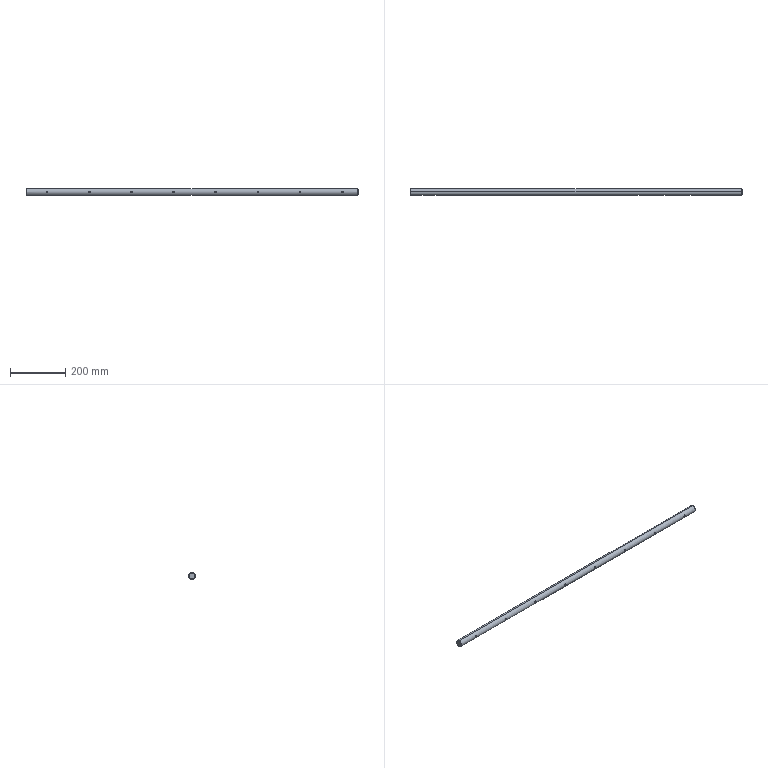Part | STEP file | 6499K55_Shaft for Support Rail_6499K55 | 1 solid | 232 faces | box 1200 x 25 x 25 mm | volume 586134 mm3 | cylinder 170 | spline 32 | cone 20 | plane 10 | commonest cylinder face diameters 6.35 x168 25 x2